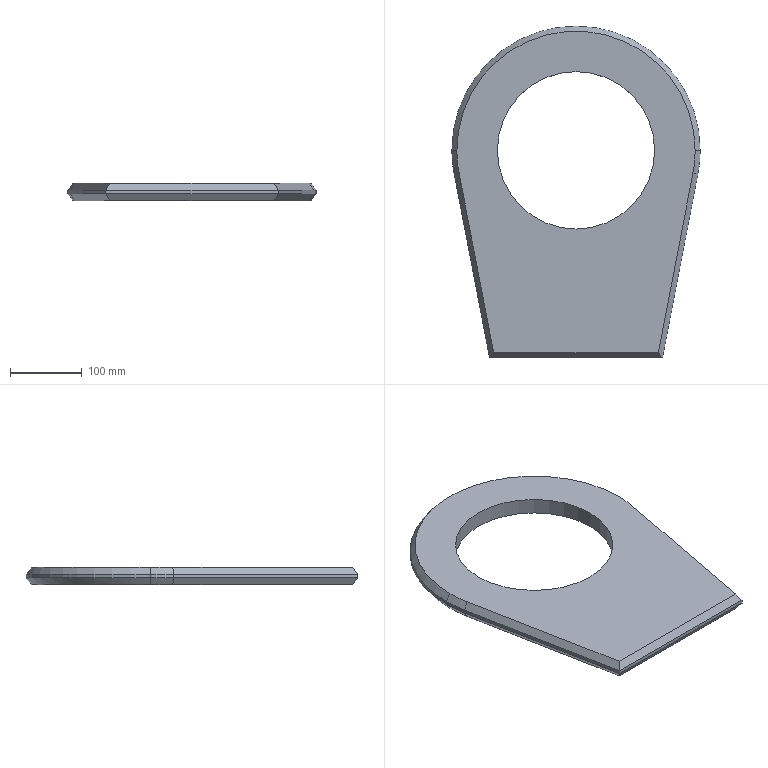Part | SolidWorks | features Chamfer 2, Extrusion 1, ICE 1 | 1 solid | 25 faces | box 347 x 463.5 x 25 mm | volume 2272890 mm3 | plane 12 | cylinder 7 | cone 6 | commonest cylinder face diameters 347 x3 220 x2 246 x2
STEP:
#1=CARTESIAN_POINT('',(166.5,290.,25.));
#2=VERTEX_POINT('',#1);
#3=CARTESIAN_POINT('',(-166.5,290.,25.));
#4=VERTEX_POINT('',#3);
#5=CARTESIAN_POINT('',(0.,290.,25.));
#6=DIRECTION('',(0.,0.,1.));
#7=DIRECTION('',(1.,0.,0.));
#8=AXIS2_PLACEMENT_3D('',#5,#6,#7);
#9=CIRCLE('',#8,166.5);
#10=EDGE_CURVE('',#2,#4,#9,.T.);
#11=ORIENTED_EDGE('',*,*,#10,.F.);
#12=CARTESIAN_POINT('',(173.5,290.,15.));
#13=VERTEX_POINT('',#12);
#14=CARTESIAN_POINT('',(166.5,290.,25.));
#15=DIRECTION('',(0.5735,0.,-0.8192));
#16=VECTOR('',#15,1000.);
#17=LINE('',#14,#16);
#18=EDGE_CURVE('',#2,#13,#17,.T.);
#19=ORIENTED_EDGE('',*,*,#18,.T.);
#20=CARTESIAN_POINT('',(-173.5,290.,15.));
#21=VERTEX_POINT('',#20);
#22=CARTESIAN_POINT('',(0.,290.,15.));
#23=DIRECTION('',(0.,0.,-1.));
#24=DIRECTION('',(1.,0.,0.));
#25=AXIS2_PLACEMENT_3D('',#22,#23,#24);
#26=CIRCLE('',#25,173.5);
#27=EDGE_CURVE('',#21,#13,#26,.T.);
#28=ORIENTED_EDGE('',*,*,#27,.F.);
#29=CARTESIAN_POINT('',(-166.5,290.,25.));
#30=DIRECTION('',(-0.5735,0.,-0.8192));
#31=VECTOR('',#30,1000.);
#32=LINE('',#29,#31);
#33=EDGE_CURVE('',#4,#21,#32,.T.);
#34=ORIENTED_EDGE('',*,*,#33,.F.);
#35=EDGE_LOOP('',(#11,#19,#28,#34));
#36=FACE_OUTER_BOUND('',#35,.T.);
#37=CARTESIAN_POINT('',(0.,290.,25.));
#38=DIRECTION('',(0.,0.,-1.));
#39=DIRECTION('',(-1.,0.,0.));
#40=AXIS2_PLACEMENT_3D('',#37,#38,#39);
#41=CONICAL_SURFACE('',#40,166.5,0.6107);
#42=ADVANCED_FACE('',(#36),#41,.T.);
#43=CARTESIAN_POINT('',(-163.497,258.52,25.));
#44=VERTEX_POINT('',#43);
#45=CARTESIAN_POINT('',(0.,290.,25.));
#46=DIRECTION('',(0.,0.,1.));
#47=DIRECTION('',(1.,0.,0.));
#48=AXIS2_PLACEMENT_3D('',#45,#46,#47);
#49=CIRCLE('',#48,166.5);
#50=EDGE_CURVE('',#4,#44,#49,.T.);
#51=ORIENTED_EDGE('',*,*,#50,.F.);
#52=ORIENTED_EDGE('',*,*,#33,.T.);
#53=CARTESIAN_POINT('',(-170.371,257.197,15.));
#54=VERTEX_POINT('',#53);
#55=CARTESIAN_POINT('',(0.,290.,15.));
#56=DIRECTION('',(0.,0.,-1.));
#57=DIRECTION('',(1.,0.,0.));
#58=AXIS2_PLACEMENT_3D('',#55,#56,#57);
#59=CIRCLE('',#58,173.5);
#60=EDGE_CURVE('',#54,#21,#59,.T.);
#61=ORIENTED_EDGE('',*,*,#60,.F.);
#62=CARTESIAN_POINT('',(-170.371,257.197,15.));
#63=DIRECTION('',(0.5631,0.1084,0.8192));
#64=VECTOR('',#63,1000.);
#65=LINE('',#62,#64);
#66=EDGE_CURVE('',#54,#44,#65,.T.);
#67=ORIENTED_EDGE('',*,*,#66,.T.);
#68=EDGE_LOOP('',(#51,#52,#61,#67));
#69=FACE_OUTER_BOUND('',#68,.T.);
#70=CARTESIAN_POINT('',(0.,290.,25.));
#71=DIRECTION('',(0.,0.,-1.));
#72=DIRECTION('',(-1.,0.,0.));
#73=AXIS2_PLACEMENT_3D('',#70,#71,#72);
#74=CONICAL_SURFACE('',#73,166.5,0.6107);
#75=ADVANCED_FACE('',(#69),#74,.T.);
#76=CARTESIAN_POINT('',(-166.5,290.,0.));
#77=VERTEX_POINT('',#76);
#78=CARTESIAN_POINT('',(166.5,290.,0.));
#79=VERTEX_POINT('',#78);
#80=CARTESIAN_POINT('',(0.,290.,0.));
#81=DIRECTION('',(0.,0.,-1.));
#82=DIRECTION('',(1.,0.,0.));
#83=AXIS2_PLACEMENT_3D('',#80,#81,#82);
#84=CIRCLE('',#83,166.5);
#85=EDGE_CURVE('',#77,#79,#84,.T.);
#86=ORIENTED_EDGE('',*,*,#85,.F.);
#87=CARTESIAN_POINT('',(-173.5,290.,10.));
#88=VERTEX_POINT('',#87);
#89=CARTESIAN_POINT('',(-173.5,290.,10.));
#90=DIRECTION('',(-0.5735,0.,0.8192));
#91=VECTOR('',#90,1000.);
#92=LINE('',#89,#91);
#93=EDGE_CURVE('',#77,#88,#92,.T.);
#94=ORIENTED_EDGE('',*,*,#93,.T.);
#95=CARTESIAN_POINT('',(173.5,290.,10.));
#96=VERTEX_POINT('',#95);
#97=CARTESIAN_POINT('',(0.,290.,10.));
#98=DIRECTION('',(0.,0.,1.));
#99=DIRECTION('',(1.,0.,0.));
#100=AXIS2_PLACEMENT_3D('',#97,#98,#99);
#101=CIRCLE('',#100,173.5);
#102=EDGE_CURVE('',#96,#88,#101,.T.);
#103=ORIENTED_EDGE('',*,*,#102,.F.);
#104=CARTESIAN_POINT('',(173.5,290.,10.));
#105=DIRECTION('',(0.5735,0.,0.8192));
#106=VECTOR('',#105,1000.);
#107=LINE('',#104,#106);
#108=EDGE_CURVE('',#79,#96,#107,.T.);
#109=ORIENTED_EDGE('',*,*,#108,.F.);
#110=EDGE_LOOP('',(#86,#94,#103,#109));
#111=FACE_OUTER_BOUND('',#110,.T.);
#112=CARTESIAN_POINT('',(0.,290.,10.));
#113=DIRECTION('',(0.,0.,1.));
#114=DIRECTION('',(1.,0.,0.));
#115=AXIS2_PLACEMENT_3D('',#112,#113,#114);
#116=CONICAL_SURFACE('',#115,173.5,0.6107);
#117=ADVANCED_FACE('',(#111),#116,.T.);
#118=CARTESIAN_POINT('',(163.497,258.52,0.));
#119=VERTEX_POINT('',#118);
#120=CARTESIAN_POINT('',(0.,290.,0.));
#121=DIRECTION('',(0.,0.,-1.));
#122=DIRECTION('',(1.,0.,0.));
#123=AXIS2_PLACEMENT_3D('',#120,#121,#122);
#124=CIRCLE('',#123,166.5);
#125=EDGE_CURVE('',#79,#119,#124,.T.);
#126=ORIENTED_EDGE('',*,*,#125,.F.);
#127=ORIENTED_EDGE('',*,*,#108,.T.);
#128=CARTESIAN_POINT('',(170.371,257.197,10.));
#129=VERTEX_POINT('',#128);
#130=CARTESIAN_POINT('',(0.,290.,10.));
#131=DIRECTION('',(0.,0.,1.));
#132=DIRECTION('',(1.,0.,0.));
#133=AXIS2_PLACEMENT_3D('',#130,#131,#132);
#134=CIRCLE('',#133,173.5);
#135=EDGE_CURVE('',#129,#96,#134,.T.);
#136=ORIENTED_EDGE('',*,*,#135,.F.);
#137=CARTESIAN_POINT('',(163.497,258.52,0.));
#138=DIRECTION('',(0.5631,-0.1084,0.8192));
#139=VECTOR('',#138,1000.);
#140=LINE('',#137,#139);
#141=EDGE_CURVE('',#119,#129,#140,.T.);
#142=ORIENTED_EDGE('',*,*,#141,.F.);
#143=EDGE_LOOP('',(#126,#127,#136,#142));
#144=FACE_OUTER_BOUND('',#143,.T.);
#145=CARTESIAN_POINT('',(0.,290.,10.));
#146=DIRECTION('',(0.,0.,1.));
#147=DIRECTION('',(1.,0.,0.));
#148=AXIS2_PLACEMENT_3D('',#145,#146,#147);
#149=CONICAL_SURFACE('',#148,173.5,0.6107);
#150=ADVANCED_FACE('',(#144),#149,.T.);
#151=CARTESIAN_POINT('',(-123.,290.,2.));
#152=VERTEX_POINT('',#151);
#153=CARTESIAN_POINT('',(123.,290.,2.));
#154=VERTEX_POINT('',#153);
#155=CARTESIAN_POINT('',(0.,290.,2.));
#156=DIRECTION('',(0.,0.,1.));
#157=DIRECTION('',(1.,0.,0.));
#158=AXIS2_PLACEMENT_3D('',#155,#156,#157);
#159=CIRCLE('',#158,123.);
#160=EDGE_CURVE('',#152,#154,#159,.T.);
#161=ORIENTED_EDGE('',*,*,#160,.T.);
#162=CARTESIAN_POINT('',(123.,290.,0.));
#163=VERTEX_POINT('',#162);
#164=CARTESIAN_POINT('',(123.,290.,2.));
#165=DIRECTION('',(0.,0.,-1.));
#166=VECTOR('',#165,1000.);
#167=LINE('',#164,#166);
#168=EDGE_CURVE('',#154,#163,#167,.T.);
#169=ORIENTED_EDGE('',*,*,#168,.T.);
#170=CARTESIAN_POINT('',(-123.,290.,0.));
#171=VERTEX_POINT('',#170);
#172=CARTESIAN_POINT('',(0.,290.,0.));
#173=DIRECTION('',(0.,0.,1.));
#174=DIRECTION('',(1.,0.,0.));
#175=AXIS2_PLACEMENT_3D('',#172,#173,#174);
#176=CIRCLE('',#175,123.);
#177=EDGE_CURVE('',#171,#163,#176,.T.);
#178=ORIENTED_EDGE('',*,*,#177,.F.);
#179=CARTESIAN_POINT('',(-123.,290.,2.));
#180=DIRECTION('',(0.,0.,-1.));
#181=VECTOR('',#180,1000.);
#182=LINE('',#179,#181);
#183=EDGE_CURVE('',#152,#171,#182,.T.);
#184=ORIENTED_EDGE('',*,*,#183,.F.);
#185=EDGE_LOOP('',(#161,#169,#178,#184));
#186=FACE_OUTER_BOUND('',#185,.T.);
#187=CARTESIAN_POINT('',(0.,290.,2.));
#188=DIRECTION('',(0.,0.,-1.));
#189=DIRECTION('',(-1.,0.,0.));
#190=AXIS2_PLACEMENT_3D('',#187,#188,#189);
#191=CYLINDRICAL_SURFACE('',#190,123.);
#192=ADVANCED_FACE('',(#186),#191,.F.);
#193=CARTESIAN_POINT('',(-110.,290.,25.));
#194=VERTEX_POINT('',#193);
#195=CARTESIAN_POINT('',(110.,290.,25.));
#196=VERTEX_POINT('',#195);
#197=CARTESIAN_POINT('',(0.,290.,25.));
#198=DIRECTION('',(0.,0.,1.));
#199=DIRECTION('',(1.,0.,0.));
#200=AXIS2_PLACEMENT_3D('',#197,#198,#199);
#201=CIRCLE('',#200,110.);
#202=EDGE_CURVE('',#194,#196,#201,.T.);
#203=ORIENTED_EDGE('',*,*,#202,.T.);
#204=CARTESIAN_POINT('',(110.,290.,2.));
#205=VERTEX_POINT('',#204);
#206=CARTESIAN_POINT('',(110.,290.,25.));
#207=DIRECTION('',(0.,0.,-1.));
#208=VECTOR('',#207,1000.);
#209=LINE('',#206,#208);
#210=EDGE_CURVE('',#196,#205,#209,.T.);
#211=ORIENTED_EDGE('',*,*,#210,.T.);
#212=CARTESIAN_POINT('',(-110.,290.,2.));
#213=VERTEX_POINT('',#212);
#214=CARTESIAN_POINT('',(0.,290.,2.));
#215=DIRECTION('',(0.,0.,1.));
#216=DIRECTION('',(1.,0.,0.));
#217=AXIS2_PLACEMENT_3D('',#214,#215,#216);
#218=CIRCLE('',#217,110.);
#219=EDGE_CURVE('',#213,#205,#218,.T.);
#220=ORIENTED_EDGE('',*,*,#219,.F.);
#221=CARTESIAN_POINT('',(-110.,290.,25.));
#222=DIRECTION('',(0.,0.,-1.));
#223=VECTOR('',#222,1000.);
#224=LINE('',#221,#223);
#225=EDGE_CURVE('',#194,#213,#224,.T.);
#226=ORIENTED_EDGE('',*,*,#225,.F.);
#227=EDGE_LOOP('',(#203,#211,#220,#226));
#228=FACE_OUTER_BOUND('',#227,.T.);
#229=CARTESIAN_POINT('',(0.,290.,25.));
#230=DIRECTION('',(0.,0.,-1.));
#231=DIRECTION('',(-1.,0.,0.));
#232=AXIS2_PLACEMENT_3D('',#229,#230,#231);
#233=CYLINDRICAL_SURFACE('',#232,110.);
#234=ADVANCED_FACE('',(#228),#233,.F.);
#235=ORIENTED_EDGE('',*,*,#27,.T.);
#236=CARTESIAN_POINT('',(173.5,290.,25.));
#237=DIRECTION('',(0.,0.,-1.));
#238=VECTOR('',#237,1000.);
#239=LINE('',#236,#238);
#240=EDGE_CURVE('',#13,#96,#239,.T.);
#241=ORIENTED_EDGE('',*,*,#240,.T.);
#242=ORIENTED_EDGE('',*,*,#102,.T.);
#243=CARTESIAN_POINT('',(-173.5,290.,25.));
#244=DIRECTION('',(0.,0.,-1.));
#245=VECTOR('',#244,1000.);
#246=LINE('',#243,#245);
#247=EDGE_CURVE('',#21,#88,#246,.T.);
#248=ORIENTED_EDGE('',*,*,#247,.F.);
#249=EDGE_LOOP('',(#235,#241,#242,#248));
#250=FACE_OUTER_BOUND('',#249,.T.);
#251=CARTESIAN_POINT('',(0.,290.,25.));
#252=DIRECTION('',(0.,0.,-1.));
#253=DIRECTION('',(-1.,0.,0.));
#254=AXIS2_PLACEMENT_3D('',#251,#252,#253);
#255=CYLINDRICAL_SURFACE('',#254,173.5);
#256=ADVANCED_FACE('',(#250),#255,.T.);
#257=ORIENTED_EDGE('',*,*,#60,.T.);
#258=ORIENTED_EDGE('',*,*,#247,.T.);
#259=CARTESIAN_POINT('',(-170.371,257.197,10.));
#260=VERTEX_POINT('',#259);
#261=CARTESIAN_POINT('',(0.,290.,10.));
#262=DIRECTION('',(0.,0.,1.));
#263=DIRECTION('',(1.,0.,0.));
#264=AXIS2_PLACEMENT_3D('',#261,#262,#263);
#265=CIRCLE('',#264,173.5);
#266=EDGE_CURVE('',#88,#260,#265,.T.);
#267=ORIENTED_EDGE('',*,*,#266,.T.);
#268=CARTESIAN_POINT('',(-170.371,257.197,25.));
#269=DIRECTION('',(0.,0.,-1.));
#270=VECTOR('',#269,1000.);
#271=LINE('',#268,#270);
#272=EDGE_CURVE('',#54,#260,#271,.T.);
#273=ORIENTED_EDGE('',*,*,#272,.F.);
#274=EDGE_LOOP('',(#257,#258,#267,#273));
#275=FACE_OUTER_BOUND('',#274,.T.);
#276=CARTESIAN_POINT('',(0.,290.,25.));
#277=DIRECTION('',(0.,0.,-1.));
#278=DIRECTION('',(-1.,0.,0.));
#279=AXIS2_PLACEMENT_3D('',#276,#277,#278);
#280=CYLINDRICAL_SURFACE('',#279,173.5);
#281=ADVANCED_FACE('',(#275),#280,.T.);
#282=CARTESIAN_POINT('',(-163.497,258.52,0.));
#283=VERTEX_POINT('',#282);
#284=CARTESIAN_POINT('',(0.,290.,0.));
#285=DIRECTION('',(0.,0.,-1.));
#286=DIRECTION('',(1.,0.,0.));
#287=AXIS2_PLACEMENT_3D('',#284,#285,#286);
#288=CIRCLE('',#287,166.5);
#289=EDGE_CURVE('',#283,#77,#288,.T.);
#290=ORIENTED_EDGE('',*,*,#289,.T.);
#291=ORIENTED_EDGE('',*,*,#85,.T.);
#292=ORIENTED_EDGE('',*,*,#125,.T.);
#293=CARTESIAN_POINT('',(115.069,7.,0.));
#294=VERTEX_POINT('',#293);
#295=CARTESIAN_POINT('',(163.497,258.52,0.));
#296=DIRECTION('',(-0.1891,-0.982,0.));
#297=VECTOR('',#296,1000.);
#298=LINE('',#295,#297);
#299=EDGE_CURVE('',#119,#294,#298,.T.);
#300=ORIENTED_EDGE('',*,*,#299,.T.);
#301=CARTESIAN_POINT('',(-115.069,7.,0.));
#302=VERTEX_POINT('',#301);
#303=CARTESIAN_POINT('',(0.,7.,0.));
#304=DIRECTION('',(-1.,0.,0.));
#305=VECTOR('',#304,1000.);
#306=LINE('',#303,#305);
#307=EDGE_CURVE('',#294,#302,#306,.T.);
#308=ORIENTED_EDGE('',*,*,#307,.T.);
#309=CARTESIAN_POINT('',(-163.497,258.52,0.));
#310=DIRECTION('',(-0.1891,0.982,0.));
#311=VECTOR('',#310,1000.);
#312=LINE('',#309,#311);
#313=EDGE_CURVE('',#302,#283,#312,.T.);
#314=ORIENTED_EDGE('',*,*,#313,.T.);
#315=EDGE_LOOP('',(#290,#291,#292,#300,#308,#314));
#316=FACE_OUTER_BOUND('',#315,.T.);
#317=ORIENTED_EDGE('',*,*,#177,.T.);
#318=CARTESIAN_POINT('',(0.,290.,0.));
#319=DIRECTION('',(0.,0.,1.));
#320=DIRECTION('',(1.,0.,0.));
#321=AXIS2_PLACEMENT_3D('',#318,#319,#320);
#322=CIRCLE('',#321,123.);
#323=EDGE_CURVE('',#163,#171,#322,.T.);
#324=ORIENTED_EDGE('',*,*,#323,.T.);
#325=EDGE_LOOP('',(#317,#324));
#326=FACE_BOUND('',#325,.T.);
#327=CARTESIAN_POINT('',(0.,290.,0.));
#328=DIRECTION('',(0.,0.,1.));
#329=DIRECTION('',(1.,0.,0.));
#330=AXIS2_PLACEMENT_3D('',#327,#328,#329);
#331=PLANE('',#330);
#332=ADVANCED_FACE('',(#316,#326),#331,.F.);
#333=CARTESIAN_POINT('',(-115.069,7.,25.));
#334=VERTEX_POINT('',#333);
#335=CARTESIAN_POINT('',(115.069,7.,25.));
#336=VERTEX_POINT('',#335);
#337=CARTESIAN_POINT('',(120.85,7.,25.));
#338=DIRECTION('',(1.,0.,0.));
#339=VECTOR('',#338,1000.);
#340=LINE('',#337,#339);
#341=EDGE_CURVE('',#334,#336,#340,.T.);
#342=ORIENTED_EDGE('',*,*,#341,.T.);
#343=CARTESIAN_POINT('',(163.497,258.52,25.));
#344=VERTEX_POINT('',#343);
#345=CARTESIAN_POINT('',(163.497,258.52,25.));
#346=DIRECTION('',(0.1891,0.982,0.));
#347=VECTOR('',#346,1000.);
#348=LINE('',#345,#347);
#349=EDGE_CURVE('',#336,#344,#348,.T.);
#350=ORIENTED_EDGE('',*,*,#349,.T.);
#351=CARTESIAN_POINT('',(0.,290.,25.));
#352=DIRECTION('',(0.,0.,1.));
#353=DIRECTION('',(1.,0.,0.));
#354=AXIS2_PLACEMENT_3D('',#351,#352,#353);
#355=CIRCLE('',#354,166.5);
#356=EDGE_CURVE('',#344,#2,#355,.T.);
#357=ORIENTED_EDGE('',*,*,#356,.T.);
#358=ORIENTED_EDGE('',*,*,#10,.T.);
#359=ORIENTED_EDGE('',*,*,#50,.T.);
#360=CARTESIAN_POINT('',(-113.976,1.323,25.));
#361=DIRECTION('',(0.1891,-0.982,0.));
#362=VECTOR('',#361,1000.);
#363=LINE('',#360,#362);
#364=EDGE_CURVE('',#44,#334,#363,.T.);
#365=ORIENTED_EDGE('',*,*,#364,.T.);
#366=EDGE_LOOP('',(#342,#350,#357,#358,#359,#365));
#367=FACE_OUTER_BOUND('',#366,.T.);
#368=ORIENTED_EDGE('',*,*,#202,.F.);
#369=CARTESIAN_POINT('',(0.,290.,25.));
#370=DIRECTION('',(0.,0.,1.));
#371=DIRECTION('',(1.,0.,0.));
#372=AXIS2_PLACEMENT_3D('',#369,#370,#371);
#373=CIRCLE('',#372,110.);
#374=EDGE_CURVE('',#196,#194,#373,.T.);
#375=ORIENTED_EDGE('',*,*,#374,.F.);
#376=EDGE_LOOP('',(#368,#375));
#377=FACE_BOUND('',#376,.T.);
#378=CARTESIAN_POINT('',(0.,290.,25.));
#379=DIRECTION('',(0.,0.,1.));
#380=DIRECTION('',(1.,0.,0.));
#381=AXIS2_PLACEMENT_3D('',#378,#379,#380);
#382=PLANE('',#381);
#383=ADVANCED_FACE('',(#367,#377),#382,.T.);
#384=CARTESIAN_POINT('',(-120.85,0.,15.));
#385=VERTEX_POINT('',#384);
#386=CARTESIAN_POINT('',(-120.85,0.,10.));
#387=VERTEX_POINT('',#386);
#388=CARTESIAN_POINT('',(-120.85,0.,25.));
#389=DIRECTION('',(0.,0.,-1.));
#390=VECTOR('',#389,1000.);
#391=LINE('',#388,#390);
#392=EDGE_CURVE('',#385,#387,#391,.T.);
#393=ORIENTED_EDGE('',*,*,#392,.F.);
#394=CARTESIAN_POINT('',(-170.371,257.197,15.));
#395=DIRECTION('',(-0.1891,0.982,0.));
#396=VECTOR('',#395,1000.);
#397=LINE('',#394,#396);
#398=EDGE_CURVE('',#385,#54,#397,.T.);
#399=ORIENTED_EDGE('',*,*,#398,.T.);
#400=ORIENTED_EDGE('',*,*,#272,.T.);
#401=CARTESIAN_POINT('',(-120.85,0.,10.));
#402=DIRECTION('',(0.1891,-0.982,0.));
#403=VECTOR('',#402,1000.);
#404=LINE('',#401,#403);
#405=EDGE_CURVE('',#260,#387,#404,.T.);
#406=ORIENTED_EDGE('',*,*,#405,.T.);
#407=EDGE_LOOP('',(#393,#399,#400,#406));
#408=FACE_OUTER_BOUND('',#407,.T.);
#409=CARTESIAN_POINT('',(-120.85,0.,25.));
#410=DIRECTION('',(0.982,0.1891,0.));
#411=DIRECTION('',(-0.1891,0.982,0.));
#412=AXIS2_PLACEMENT_3D('',#409,#410,#411);
#413=PLANE('',#412);
#414=ADVANCED_FACE('',(#408),#413,.F.);
#415=CARTESIAN_POINT('',(120.85,0.,15.));
#416=VERTEX_POINT('',#415);
#417=CARTESIAN_POINT('',(120.85,0.,10.));
#418=VERTEX_POINT('',#417);
#419=CARTESIAN_POINT('',(120.85,0.,25.));
#420=DIRECTION('',(0.,0.,-1.));
#421=VECTOR('',#420,1000.);
#422=LINE('',#419,#421);
#423=EDGE_CURVE('',#416,#418,#422,.T.);
#424=ORIENTED_EDGE('',*,*,#423,.F.);
#425=CARTESIAN_POINT('',(-120.85,0.,15.));
#426=DIRECTION('',(-1.,0.,0.));
#427=VECTOR('',#426,1000.);
#428=LINE('',#425,#427);
#429=EDGE_CURVE('',#416,#385,#428,.T.);
#430=ORIENTED_EDGE('',*,*,#429,.T.);
#431=ORIENTED_EDGE('',*,*,#392,.T.);
#432=CARTESIAN_POINT('',(-120.85,0.,10.));
#433=DIRECTION('',(1.,0.,0.));
#434=VECTOR('',#433,1000.);
#435=LINE('',#432,#434);
#436=EDGE_CURVE('',#387,#418,#435,.T.);
#437=ORIENTED_EDGE('',*,*,#436,.T.);
#438=EDGE_LOOP('',(#424,#430,#431,#437));
#439=FACE_OUTER_BOUND('',#438,.T.);
#440=CARTESIAN_POINT('',(-120.85,0.,25.));
#441=DIRECTION('',(0.,1.,0.));
#442=DIRECTION('',(0.,0.,1.));
#443=AXIS2_PLACEMENT_3D('',#440,#441,#442);
#444=PLANE('',#443);
#445=ADVANCED_FACE('',(#439),#444,.F.);
#446=CARTESIAN_POINT('',(170.371,257.197,15.));
#447=VERTEX_POINT('',#446);
#448=CARTESIAN_POINT('',(170.371,257.197,25.));
#449=DIRECTION('',(0.,0.,-1.));
#450=VECTOR('',#449,1000.);
#451=LINE('',#448,#450);
#452=EDGE_CURVE('',#447,#129,#451,.T.);
#453=ORIENTED_EDGE('',*,*,#452,.F.);
#454=CARTESIAN_POINT('',(120.85,0.,15.));
#455=DIRECTION('',(-0.1891,-0.982,0.));
#456=VECTOR('',#455,1000.);
#457=LINE('',#454,#456);
#458=EDGE_CURVE('',#447,#416,#457,.T.);
#459=ORIENTED_EDGE('',*,*,#458,.T.);
#460=ORIENTED_EDGE('',*,*,#423,.T.);
#461=CARTESIAN_POINT('',(120.85,0.,10.));
#462=DIRECTION('',(0.1891,0.982,0.));
#463=VECTOR('',#462,1000.);
#464=LINE('',#461,#463);
#465=EDGE_CURVE('',#418,#129,#464,.T.);
#466=ORIENTED_EDGE('',*,*,#465,.T.);
#467=EDGE_LOOP('',(#453,#459,#460,#466));
#468=FACE_OUTER_BOUND('',#467,.T.);
#469=CARTESIAN_POINT('',(120.85,0.,25.));
#470=DIRECTION('',(-0.982,0.1891,0.));
#471=DIRECTION('',(-0.1891,-0.982,0.));
#472=AXIS2_PLACEMENT_3D('',#469,#470,#471);
#473=PLANE('',#472);
#474=ADVANCED_FACE('',(#468),#473,.F.);
#475=ORIENTED_EDGE('',*,*,#240,.F.);
#476=CARTESIAN_POINT('',(0.,290.,15.));
#477=DIRECTION('',(0.,0.,-1.));
#478=DIRECTION('',(1.,0.,0.));
#479=AXIS2_PLACEMENT_3D('',#476,#477,#478);
#480=CIRCLE('',#479,173.5);
#481=EDGE_CURVE('',#13,#447,#480,.T.);
#482=ORIENTED_EDGE('',*,*,#481,.T.);
#483=ORIENTED_EDGE('',*,*,#452,.T.);
#484=ORIENTED_EDGE('',*,*,#135,.T.);
#485=EDGE_LOOP('',(#475,#482,#483,#484));
#486=FACE_OUTER_BOUND('',#485,.T.);
#487=CARTESIAN_POINT('',(0.,290.,25.));
#488=DIRECTION('',(0.,0.,-1.));
#489=DIRECTION('',(-1.,0.,0.));
#490=AXIS2_PLACEMENT_3D('',#487,#488,#489);
#491=CYLINDRICAL_SURFACE('',#490,173.5);
#492=ADVANCED_FACE('',(#486),#491,.T.);
#493=ORIENTED_EDGE('',*,*,#210,.F.);
#494=ORIENTED_EDGE('',*,*,#374,.T.);
#495=ORIENTED_EDGE('',*,*,#225,.T.);
#496=CARTESIAN_POINT('',(0.,290.,2.));
#497=DIRECTION('',(0.,0.,1.));
#498=DIRECTION('',(1.,0.,0.));
#499=AXIS2_PLACEMENT_3D('',#496,#497,#498);
#500=CIRCLE('',#499,110.);
#501=EDGE_CURVE('',#205,#213,#500,.T.);
#502=ORIENTED_EDGE('',*,*,#501,.F.);
#503=EDGE_LOOP('',(#493,#494,#495,#502));
#504=FACE_OUTER_BOUND('',#503,.T.);
#505=CARTESIAN_POINT('',(0.,290.,25.));
#506=DIRECTION('',(0.,0.,-1.));
#507=DIRECTION('',(-1.,0.,0.));
#508=AXIS2_PLACEMENT_3D('',#505,#506,#507);
#509=CYLINDRICAL_SURFACE('',#508,110.);
#510=ADVANCED_FACE('',(#504),#509,.F.);
#511=ORIENTED_EDGE('',*,*,#160,.F.);
#512=CARTESIAN_POINT('',(0.,290.,2.));
#513=DIRECTION('',(0.,0.,1.));
#514=DIRECTION('',(1.,0.,0.));
#515=AXIS2_PLACEMENT_3D('',#512,#513,#514);
#516=CIRCLE('',#515,123.);
#517=EDGE_CURVE('',#154,#152,#516,.T.);
#518=ORIENTED_EDGE('',*,*,#517,.F.);
#519=EDGE_LOOP('',(#511,#518));
#520=FACE_OUTER_BOUND('',#519,.T.);
#521=ORIENTED_EDGE('',*,*,#219,.T.);
#522=ORIENTED_EDGE('',*,*,#501,.T.);
#523=EDGE_LOOP('',(#521,#522));
#524=FACE_BOUND('',#523,.T.);
#525=CARTESIAN_POINT('',(0.,290.,2.));
#526=DIRECTION('',(0.,0.,1.));
#527=DIRECTION('',(1.,0.,0.));
#528=AXIS2_PLACEMENT_3D('',#525,#526,#527);
#529=PLANE('',#528);
#530=ADVANCED_FACE('',(#520,#524),#529,.F.);
#531=ORIENTED_EDGE('',*,*,#168,.F.);
#532=ORIENTED_EDGE('',*,*,#517,.T.);
#533=ORIENTED_EDGE('',*,*,#183,.T.);
#534=ORIENTED_EDGE('',*,*,#323,.F.);
#535=EDGE_LOOP('',(#531,#532,#533,#534));
#536=FACE_OUTER_BOUND('',#535,.T.);
#537=CARTESIAN_POINT('',(0.,290.,2.));
#538=DIRECTION('',(0.,0.,-1.));
#539=DIRECTION('',(-1.,0.,0.));
#540=AXIS2_PLACEMENT_3D('',#537,#538,#539);
#541=CYLINDRICAL_SURFACE('',#540,123.);
#542=ADVANCED_FACE('',(#536),#541,.F.);
#543=CARTESIAN_POINT('',(-163.497,258.52,0.));
#544=DIRECTION('',(-0.5631,-0.1084,0.8192));
#545=VECTOR('',#544,1000.);
#546=LINE('',#543,#545);
#547=EDGE_CURVE('',#283,#260,#546,.T.);
#548=ORIENTED_EDGE('',*,*,#547,.F.);
#549=ORIENTED_EDGE('',*,*,#313,.F.);
#550=CARTESIAN_POINT('',(-120.85,0.,10.));
#551=DIRECTION('',(0.428,0.5183,-0.7404));
#552=VECTOR('',#551,1000.);
#553=LINE('',#550,#552);
#554=EDGE_CURVE('',#387,#302,#553,.T.);
#555=ORIENTED_EDGE('',*,*,#554,.F.);
#556=ORIENTED_EDGE('',*,*,#405,.F.);
#557=EDGE_LOOP('',(#548,#549,#555,#556));
#558=FACE_OUTER_BOUND('',#557,.T.);
#559=CARTESIAN_POINT('',(-120.85,0.,10.));
#560=DIRECTION('',(0.8045,0.1549,0.5735));
#561=DIRECTION('',(0.5805,0.,-0.8143));
#562=AXIS2_PLACEMENT_3D('',#559,#560,#561);
#563=PLANE('',#562);
#564=ADVANCED_FACE('',(#558),#563,.F.);
#565=ORIENTED_EDGE('',*,*,#554,.T.);
#566=ORIENTED_EDGE('',*,*,#307,.F.);
#567=CARTESIAN_POINT('',(76.572,53.616,-66.594));
#568=DIRECTION('',(-0.428,0.5183,-0.7404));
#569=VECTOR('',#568,1000.);
#570=LINE('',#567,#569);
#571=EDGE_CURVE('',#418,#294,#570,.T.);
#572=ORIENTED_EDGE('',*,*,#571,.F.);
#573=ORIENTED_EDGE('',*,*,#436,.F.);
#574=EDGE_LOOP('',(#565,#566,#572,#573));
#575=FACE_OUTER_BOUND('',#574,.T.);
#576=CARTESIAN_POINT('',(-120.85,0.,10.));
#577=DIRECTION('',(0.,0.8192,0.5735));
#578=DIRECTION('',(0.,-0.5735,0.8192));
#579=AXIS2_PLACEMENT_3D('',#576,#577,#578);
#580=PLANE('',#579);
#581=ADVANCED_FACE('',(#575),#580,.F.);
#582=ORIENTED_EDGE('',*,*,#93,.F.);
#583=ORIENTED_EDGE('',*,*,#289,.F.);
#584=ORIENTED_EDGE('',*,*,#547,.T.);
#585=ORIENTED_EDGE('',*,*,#266,.F.);
#586=EDGE_LOOP('',(#582,#583,#584,#585));
#587=FACE_OUTER_BOUND('',#586,.T.);
#588=CARTESIAN_POINT('',(0.,290.,10.));
#589=DIRECTION('',(0.,0.,1.));
#590=DIRECTION('',(1.,0.,0.));
#591=AXIS2_PLACEMENT_3D('',#588,#589,#590);
#592=CONICAL_SURFACE('',#591,173.5,0.6107);
#593=ADVANCED_FACE('',(#587),#592,.T.);
#594=ORIENTED_EDGE('',*,*,#571,.T.);
#595=ORIENTED_EDGE('',*,*,#299,.F.);
#596=ORIENTED_EDGE('',*,*,#141,.T.);
#597=ORIENTED_EDGE('',*,*,#465,.F.);
#598=EDGE_LOOP('',(#594,#595,#596,#597));
#599=FACE_OUTER_BOUND('',#598,.T.);
#600=CARTESIAN_POINT('',(120.85,0.,10.));
#601=DIRECTION('',(-0.8045,0.1549,0.5735));
#602=DIRECTION('',(0.5805,0.,0.8143));
#603=AXIS2_PLACEMENT_3D('',#600,#601,#602);
#604=PLANE('',#603);
#605=ADVANCED_FACE('',(#599),#604,.F.);
#606=ORIENTED_EDGE('',*,*,#66,.F.);
#607=ORIENTED_EDGE('',*,*,#398,.F.);
#608=CARTESIAN_POINT('',(-93.989,32.526,61.465));
#609=DIRECTION('',(-0.428,-0.5183,-0.7404));
#610=VECTOR('',#609,1000.);
#611=LINE('',#608,#610);
#612=EDGE_CURVE('',#334,#385,#611,.T.);
#613=ORIENTED_EDGE('',*,*,#612,.F.);
#614=ORIENTED_EDGE('',*,*,#364,.F.);
#615=EDGE_LOOP('',(#606,#607,#613,#614));
#616=FACE_OUTER_BOUND('',#615,.T.);
#617=CARTESIAN_POINT('',(-163.497,258.52,25.));
#618=DIRECTION('',(-0.8045,-0.1549,0.5735));
#619=DIRECTION('',(0.5805,0.,0.8143));
#620=AXIS2_PLACEMENT_3D('',#617,#618,#619);
#621=PLANE('',#620);
#622=ADVANCED_FACE('',(#616),#621,.T.);
#623=ORIENTED_EDGE('',*,*,#612,.T.);
#624=ORIENTED_EDGE('',*,*,#429,.F.);
#625=CARTESIAN_POINT('',(93.989,32.526,61.465));
#626=DIRECTION('',(0.428,-0.5183,-0.7404));
#627=VECTOR('',#626,1000.);
#628=LINE('',#625,#627);
#629=EDGE_CURVE('',#336,#416,#628,.T.);
#630=ORIENTED_EDGE('',*,*,#629,.F.);
#631=ORIENTED_EDGE('',*,*,#341,.F.);
#632=EDGE_LOOP('',(#623,#624,#630,#631));
#633=FACE_OUTER_BOUND('',#632,.T.);
#634=CARTESIAN_POINT('',(0.,7.,25.));
#635=DIRECTION('',(0.,-0.8192,0.5735));
#636=DIRECTION('',(0.,-0.5735,-0.8192));
#637=AXIS2_PLACEMENT_3D('',#634,#635,#636);
#638=PLANE('',#637);
#639=ADVANCED_FACE('',(#633),#638,.T.);
#640=ORIENTED_EDGE('',*,*,#18,.F.);
#641=ORIENTED_EDGE('',*,*,#356,.F.);
#642=CARTESIAN_POINT('',(170.371,257.197,15.));
#643=DIRECTION('',(-0.5631,0.1084,0.8192));
#644=VECTOR('',#643,1000.);
#645=LINE('',#642,#644);
#646=EDGE_CURVE('',#447,#344,#645,.T.);
#647=ORIENTED_EDGE('',*,*,#646,.F.);
#648=ORIENTED_EDGE('',*,*,#481,.F.);
#649=EDGE_LOOP('',(#640,#641,#647,#648));
#650=FACE_OUTER_BOUND('',#649,.T.);
#651=CARTESIAN_POINT('',(0.,290.,25.));
#652=DIRECTION('',(0.,0.,-1.));
#653=DIRECTION('',(-1.,0.,0.));
#654=AXIS2_PLACEMENT_3D('',#651,#652,#653);
#655=CONICAL_SURFACE('',#654,166.5,0.6107);
#656=ADVANCED_FACE('',(#650),#655,.T.);
#657=ORIENTED_EDGE('',*,*,#629,.T.);
#658=ORIENTED_EDGE('',*,*,#458,.F.);
#659=ORIENTED_EDGE('',*,*,#646,.T.);
#660=ORIENTED_EDGE('',*,*,#349,.F.);
#661=EDGE_LOOP('',(#657,#658,#659,#660));
#662=FACE_OUTER_BOUND('',#661,.T.);
#663=CARTESIAN_POINT('',(163.497,258.52,25.));
#664=DIRECTION('',(0.8045,-0.1549,0.5735));
#665=DIRECTION('',(0.5805,0.,-0.8143));
#666=AXIS2_PLACEMENT_3D('',#663,#664,#665);
#667=PLANE('',#666);
#668=ADVANCED_FACE('',(#662),#667,.T.);
#669=CLOSED_SHELL('',(#42,#75,#117,#150,#192,#234,#256,#281,#332,#383,#414,#445,#474,#492,#510,#530,#542,#564,#581,#593,#605,#622,#639,#656,#668));
#670=MANIFOLD_SOLID_BREP('',#669);
#671=CARTESIAN_POINT('',(0.,0.,0.));
#672=DIRECTION('',(0.,0.,1.));
#673=DIRECTION('',(1.,0.,0.));
#674=AXIS2_PLACEMENT_3D('',#671,#672,#673);
#675=(LENGTH_UNIT()NAMED_UNIT(*)SI_UNIT(.MILLI.,.METRE.));
#676=UNCERTAINTY_MEASURE_WITH_UNIT(LENGTH_MEASURE(0.00001),#675,'','');
#677=(NAMED_UNIT(*)PLANE_ANGLE_UNIT()SI_UNIT($,.RADIAN.));
#678=(NAMED_UNIT(*)SI_UNIT($,.STERADIAN.)SOLID_ANGLE_UNIT());
#679=(GEOMETRIC_REPRESENTATION_CONTEXT(3)GLOBAL_UNCERTAINTY_ASSIGNED_CONTEXT((#676))GLOBAL_UNIT_ASSIGNED_CONTEXT((#675,#677,#678))REPRESENTATION_CONTEXT('',''));
#680=ADVANCED_BREP_SHAPE_REPRESENTATION('',(#670,#674),#679);